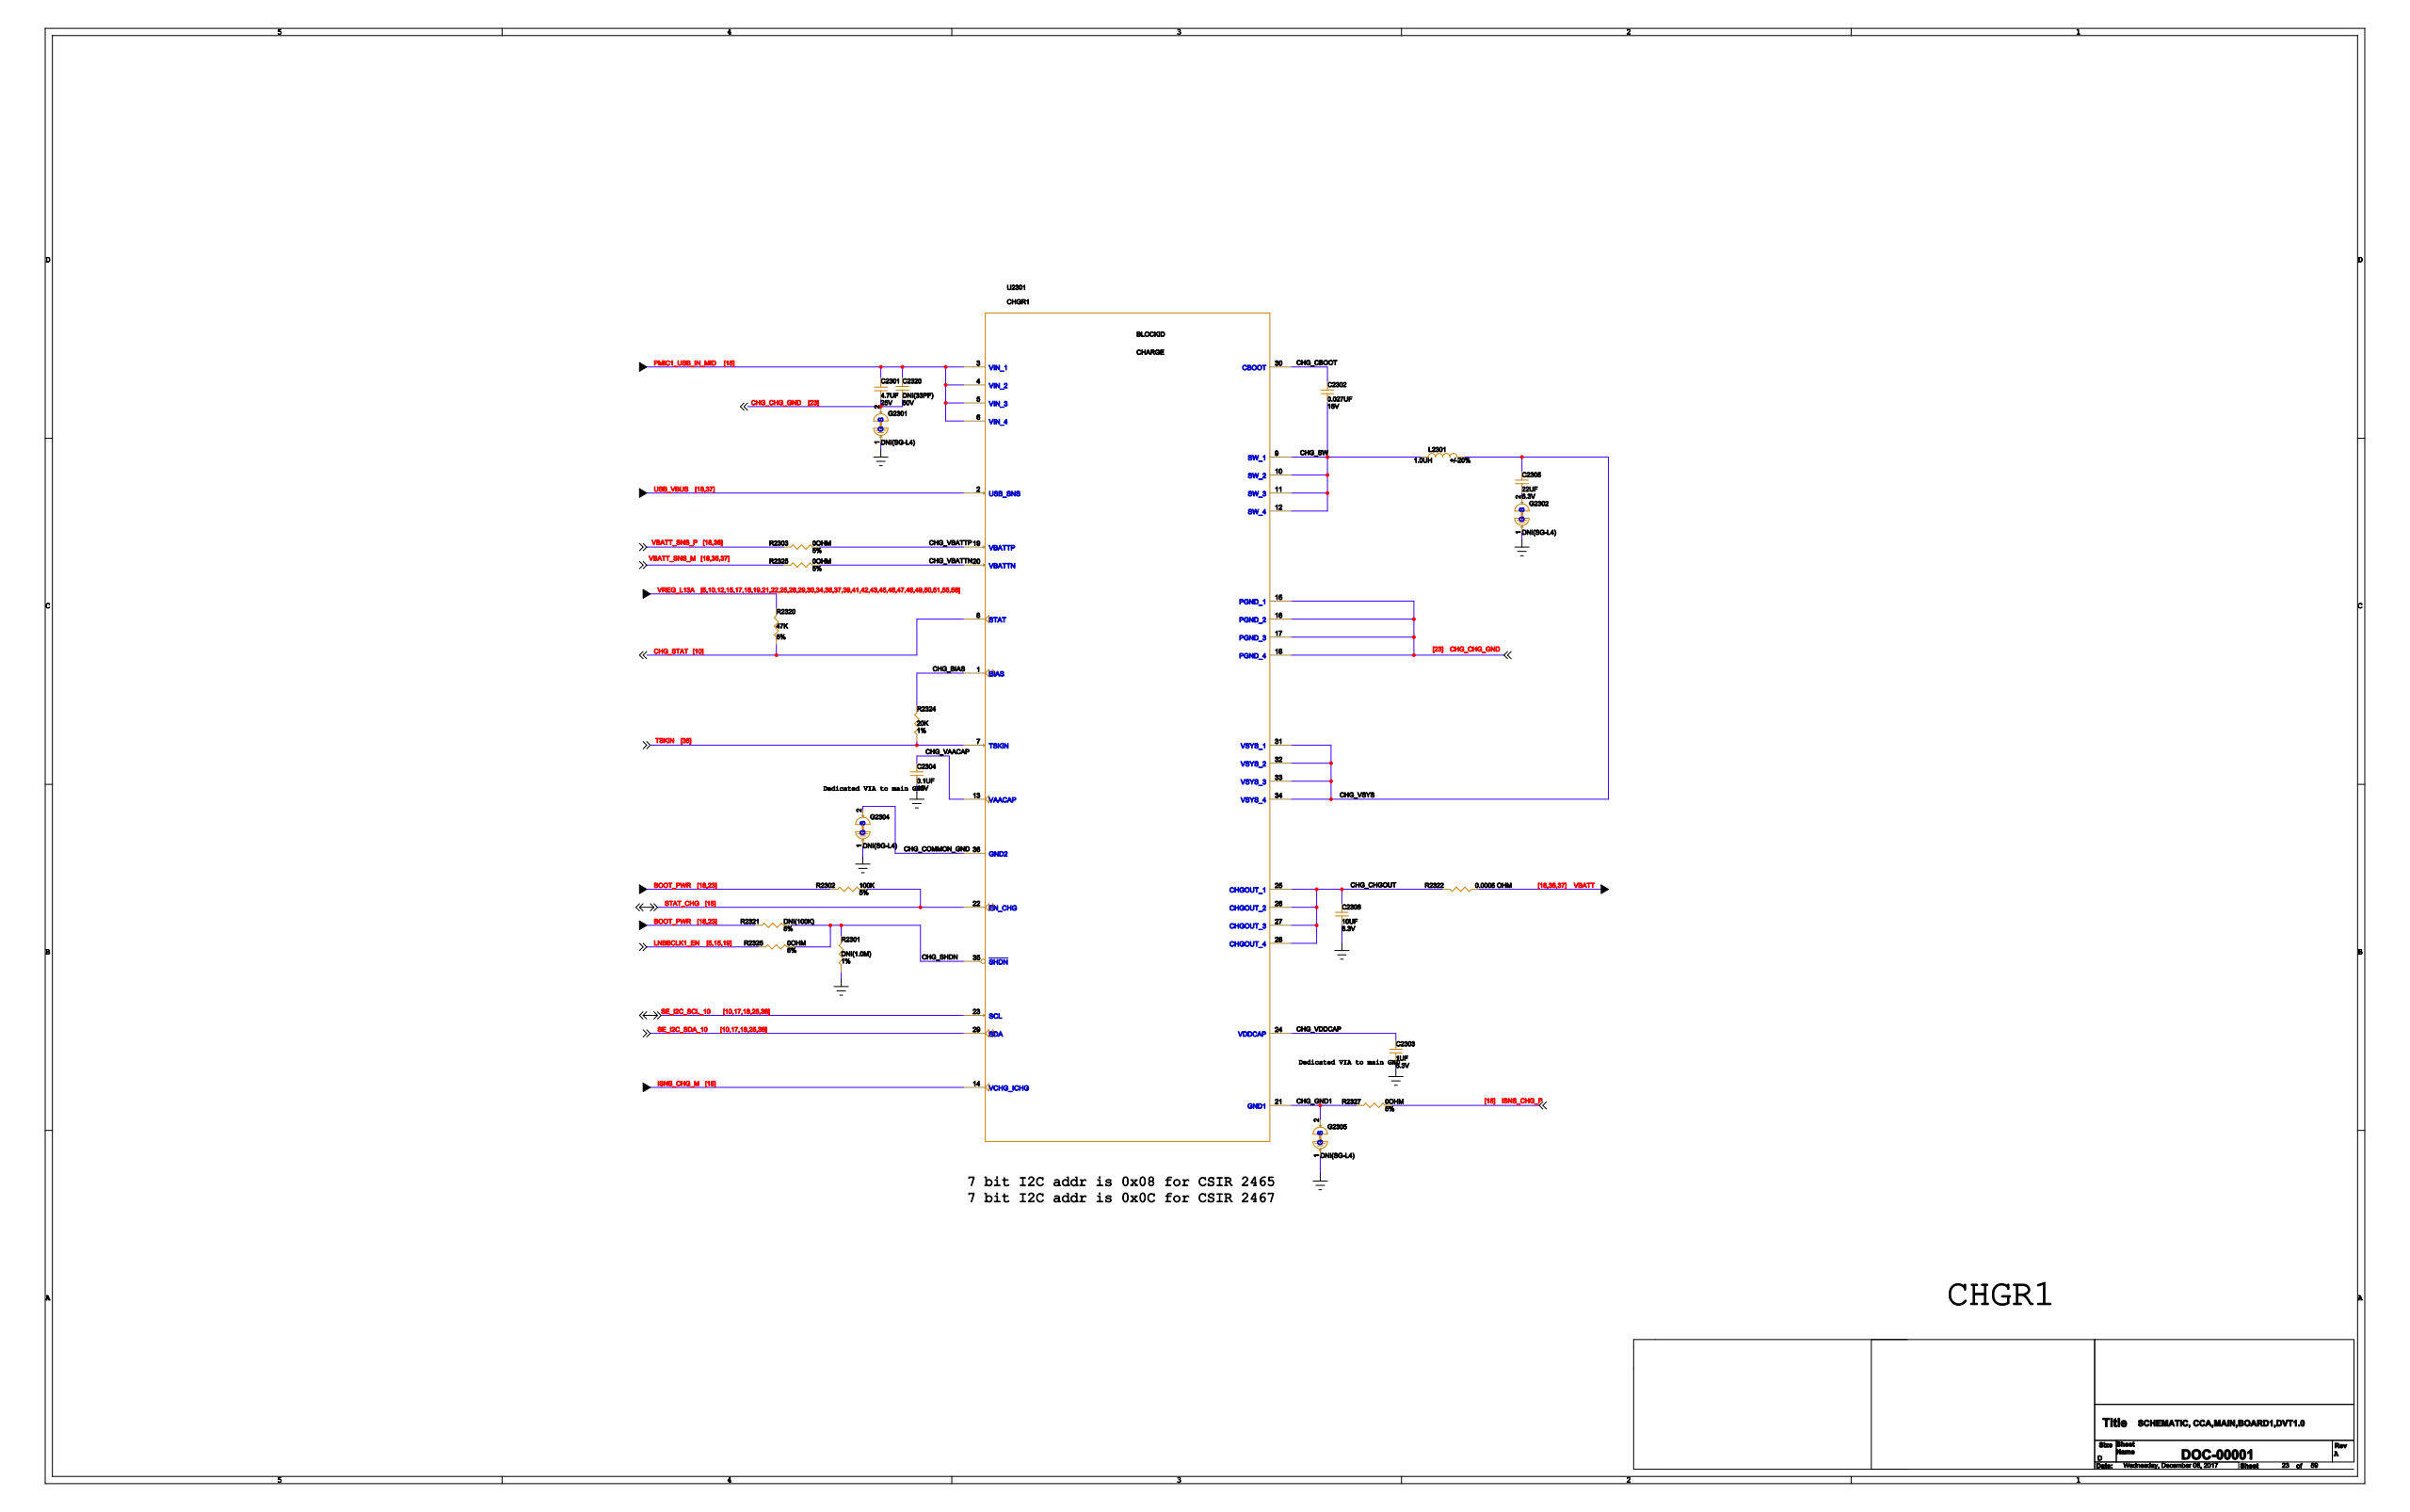Circuit board | KiCad | 1657 parts | 1365 nets | one sheet of the schematic
Parts on this sheet (reference | value | footprint):
C2301
C2302
C2303
C2304
C2305
C2306
C2320
G2301
G2302
G2304
G2305
L2301
R2301
R2302
R2303
R2320
R2321
R2322
R2324
R2325
R2326
R2327
U2301
Nets of these parts (net: part-pin ...):
GND: C2303-2 C2304-2 C2306-2 G2301-1 G2302-1 G2304-1 G2305-1 R2301-2
VREG_L13A: R2320-1
VBATT_SNS_P: R2303-1
CHG_VBATTP: R2303-2 U2301-19
CHG_CHG_GND: C2301-1 C2320-2 G2301-2 U2301-15 U2301-16 U2301-17 U2301-18
IC1_USB_IN_MID: C2301-2 C2320-1 U2301-3 U2301-4 U2301-5 U2301-6
LNBBCLK1_EN: R2326-1
CHG_GND1: G2305-2 R2327-1 U2301-21
BOOT_PWR: R2302-1 R2321-1
STAT_CHG: R2302-2 U2301-22
CHG_BIAS: R2324-1 U2301-1
TSKIN: R2324-2 U2301-7
USB_VBUS: U2301-2
SE_I2C_SCL_10: U2301-23
SE_I2C_SDA_10: U2301-29
CHG_VAACAP: C2304-1 U2301-13
CHG_SHDN: R2301-1 R2321-2 R2326-2 U2301-35
VBATT: R2322-2
CHG_CBOOT: C2302-1 U2301-30
CHG_SW: C2302-2 L2301-1 U2301-9 U2301-10 U2301-11 U2301-12
VBATT_SNS_M: R2325-1
CHG_CHGOUT: C2306-1 R2322-1 U2301-25 U2301-26 U2301-27 U2301-28
CHG_STAT: R2320-2 U2301-8
ISNS_CHG_M: U2301-14
CHG_VBATTN: R2325-2 U2301-20
CHG_VDDCAP: C2303-1 U2301-24
CHG_VSYS: C2305-1 L2301-2 U2301-31 U2301-32 U2301-33 U2301-34
CHG_COMMON_GND: G2304-2 U2301-36
N22444153: C2305-2 G2302-2
ISNS_CHG_P: R2327-2